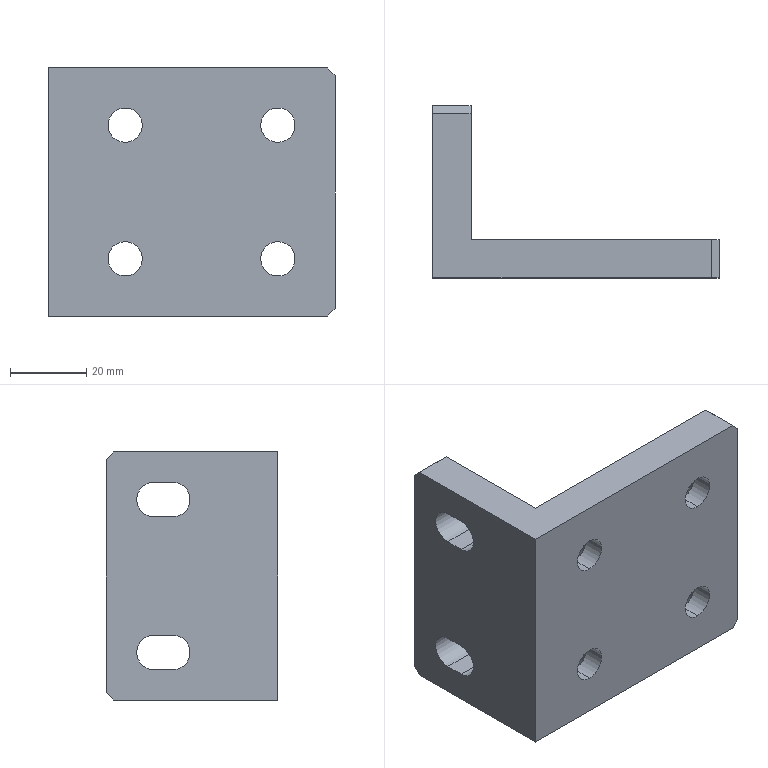Part | SolidWorks | features ICE 2, Chamfer 1, Extrusion 1, HoleWzd 1 | 1 solid | 36 faces | box 75 x 45 x 65 mm | volume 65207 mm3 | plane 16 | cylinder 12 | cone 8 | commonest cylinder face diameters 9 x12
STEP:
#1=CARTESIAN_POINT('',(22.5,0.54,-22.));
#2=VERTEX_POINT('',#1);
#3=CARTESIAN_POINT('',(22.5,0.54,-13.));
#4=VERTEX_POINT('',#3);
#5=CARTESIAN_POINT('',(22.5,0.54,-17.5));
#6=DIRECTION('',(0.,1.,0.));
#7=DIRECTION('',(0.,0.,1.));
#8=AXIS2_PLACEMENT_3D('',#5,#6,#7);
#9=CIRCLE('',#8,4.5);
#10=EDGE_CURVE('',#2,#4,#9,.T.);
#11=ORIENTED_EDGE('',*,*,#10,.F.);
#12=CARTESIAN_POINT('',(22.5,5.,-26.46));
#13=VERTEX_POINT('',#12);
#14=CARTESIAN_POINT('',(22.5,5.,-26.46));
#15=DIRECTION('',(0.,0.7071,-0.7071));
#16=VECTOR('',#15,1000.);
#17=LINE('',#14,#16);
#18=EDGE_CURVE('',#2,#13,#17,.T.);
#19=ORIENTED_EDGE('',*,*,#18,.T.);
#20=CARTESIAN_POINT('',(22.5,5.,-8.54));
#21=VERTEX_POINT('',#20);
#22=CARTESIAN_POINT('',(22.5,5.,-17.5));
#23=DIRECTION('',(0.,1.,0.));
#24=DIRECTION('',(0.,0.,1.));
#25=AXIS2_PLACEMENT_3D('',#22,#23,#24);
#26=CIRCLE('',#25,8.96);
#27=EDGE_CURVE('',#13,#21,#26,.T.);
#28=ORIENTED_EDGE('',*,*,#27,.T.);
#29=CARTESIAN_POINT('',(22.5,5.,-8.54));
#30=DIRECTION('',(0.,0.7071,0.7071));
#31=VECTOR('',#30,1000.);
#32=LINE('',#29,#31);
#33=EDGE_CURVE('',#4,#21,#32,.T.);
#34=ORIENTED_EDGE('',*,*,#33,.F.);
#35=EDGE_LOOP('',(#11,#19,#28,#34));
#36=FACE_OUTER_BOUND('',#35,.T.);
#37=CARTESIAN_POINT('',(22.5,5.,-17.5));
#38=DIRECTION('',(0.,1.,0.));
#39=DIRECTION('',(0.,0.,1.));
#40=AXIS2_PLACEMENT_3D('',#37,#38,#39);
#41=CONICAL_SURFACE('',#40,8.96,0.7854);
#42=ADVANCED_FACE('',(#36),#41,.F.);
#43=CARTESIAN_POINT('',(22.5,-5.,-22.));
#44=VERTEX_POINT('',#43);
#45=CARTESIAN_POINT('',(22.5,-5.,-13.));
#46=VERTEX_POINT('',#45);
#47=CARTESIAN_POINT('',(22.5,-5.,-17.5));
#48=DIRECTION('',(0.,1.,0.));
#49=DIRECTION('',(0.,0.,1.));
#50=AXIS2_PLACEMENT_3D('',#47,#48,#49);
#51=CIRCLE('',#50,4.5);
#52=EDGE_CURVE('',#44,#46,#51,.T.);
#53=ORIENTED_EDGE('',*,*,#52,.F.);
#54=CARTESIAN_POINT('',(22.5,5.,-22.));
#55=DIRECTION('',(0.,1.,0.));
#56=VECTOR('',#55,1000.);
#57=LINE('',#54,#56);
#58=EDGE_CURVE('',#44,#2,#57,.T.);
#59=ORIENTED_EDGE('',*,*,#58,.T.);
#60=ORIENTED_EDGE('',*,*,#10,.T.);
#61=CARTESIAN_POINT('',(22.5,5.,-13.));
#62=DIRECTION('',(0.,1.,0.));
#63=VECTOR('',#62,1000.);
#64=LINE('',#61,#63);
#65=EDGE_CURVE('',#46,#4,#64,.T.);
#66=ORIENTED_EDGE('',*,*,#65,.F.);
#67=EDGE_LOOP('',(#53,#59,#60,#66));
#68=FACE_OUTER_BOUND('',#67,.T.);
#69=CARTESIAN_POINT('',(22.5,5.,-17.5));
#70=DIRECTION('',(0.,1.,0.));
#71=DIRECTION('',(0.,0.,1.));
#72=AXIS2_PLACEMENT_3D('',#69,#70,#71);
#73=CYLINDRICAL_SURFACE('',#72,4.5);
#74=ADVANCED_FACE('',(#68),#73,.F.);
#75=CARTESIAN_POINT('',(-17.5,0.54,-22.));
#76=VERTEX_POINT('',#75);
#77=CARTESIAN_POINT('',(-17.5,0.54,-13.));
#78=VERTEX_POINT('',#77);
#79=CARTESIAN_POINT('',(-17.5,0.54,-17.5));
#80=DIRECTION('',(0.,1.,0.));
#81=DIRECTION('',(0.,0.,1.));
#82=AXIS2_PLACEMENT_3D('',#79,#80,#81);
#83=CIRCLE('',#82,4.5);
#84=EDGE_CURVE('',#76,#78,#83,.T.);
#85=ORIENTED_EDGE('',*,*,#84,.F.);
#86=CARTESIAN_POINT('',(-17.5,5.,-26.46));
#87=VERTEX_POINT('',#86);
#88=CARTESIAN_POINT('',(-17.5,5.,-26.46));
#89=DIRECTION('',(0.,0.7071,-0.7071));
#90=VECTOR('',#89,1000.);
#91=LINE('',#88,#90);
#92=EDGE_CURVE('',#76,#87,#91,.T.);
#93=ORIENTED_EDGE('',*,*,#92,.T.);
#94=CARTESIAN_POINT('',(-17.5,5.,-8.54));
#95=VERTEX_POINT('',#94);
#96=CARTESIAN_POINT('',(-17.5,5.,-17.5));
#97=DIRECTION('',(0.,1.,0.));
#98=DIRECTION('',(0.,0.,1.));
#99=AXIS2_PLACEMENT_3D('',#96,#97,#98);
#100=CIRCLE('',#99,8.96);
#101=EDGE_CURVE('',#87,#95,#100,.T.);
#102=ORIENTED_EDGE('',*,*,#101,.T.);
#103=CARTESIAN_POINT('',(-17.5,5.,-8.54));
#104=DIRECTION('',(0.,0.7071,0.7071));
#105=VECTOR('',#104,1000.);
#106=LINE('',#103,#105);
#107=EDGE_CURVE('',#78,#95,#106,.T.);
#108=ORIENTED_EDGE('',*,*,#107,.F.);
#109=EDGE_LOOP('',(#85,#93,#102,#108));
#110=FACE_OUTER_BOUND('',#109,.T.);
#111=CARTESIAN_POINT('',(-17.5,5.,-17.5));
#112=DIRECTION('',(0.,1.,0.));
#113=DIRECTION('',(0.,0.,1.));
#114=AXIS2_PLACEMENT_3D('',#111,#112,#113);
#115=CONICAL_SURFACE('',#114,8.96,0.7854);
#116=ADVANCED_FACE('',(#110),#115,.F.);
#117=CARTESIAN_POINT('',(-17.5,-5.,-22.));
#118=VERTEX_POINT('',#117);
#119=CARTESIAN_POINT('',(-17.5,-5.,-13.));
#120=VERTEX_POINT('',#119);
#121=CARTESIAN_POINT('',(-17.5,-5.,-17.5));
#122=DIRECTION('',(0.,1.,0.));
#123=DIRECTION('',(0.,0.,1.));
#124=AXIS2_PLACEMENT_3D('',#121,#122,#123);
#125=CIRCLE('',#124,4.5);
#126=EDGE_CURVE('',#118,#120,#125,.T.);
#127=ORIENTED_EDGE('',*,*,#126,.F.);
#128=CARTESIAN_POINT('',(-17.5,5.,-22.));
#129=DIRECTION('',(0.,1.,0.));
#130=VECTOR('',#129,1000.);
#131=LINE('',#128,#130);
#132=EDGE_CURVE('',#118,#76,#131,.T.);
#133=ORIENTED_EDGE('',*,*,#132,.T.);
#134=ORIENTED_EDGE('',*,*,#84,.T.);
#135=CARTESIAN_POINT('',(-17.5,5.,-13.));
#136=DIRECTION('',(0.,1.,0.));
#137=VECTOR('',#136,1000.);
#138=LINE('',#135,#137);
#139=EDGE_CURVE('',#120,#78,#138,.T.);
#140=ORIENTED_EDGE('',*,*,#139,.F.);
#141=EDGE_LOOP('',(#127,#133,#134,#140));
#142=FACE_OUTER_BOUND('',#141,.T.);
#143=CARTESIAN_POINT('',(-17.5,5.,-17.5));
#144=DIRECTION('',(0.,1.,0.));
#145=DIRECTION('',(0.,0.,1.));
#146=AXIS2_PLACEMENT_3D('',#143,#144,#145);
#147=CYLINDRICAL_SURFACE('',#146,4.5);
#148=ADVANCED_FACE('',(#142),#147,.F.);
#149=CARTESIAN_POINT('',(-17.5,0.54,13.));
#150=VERTEX_POINT('',#149);
#151=CARTESIAN_POINT('',(-17.5,0.54,22.));
#152=VERTEX_POINT('',#151);
#153=CARTESIAN_POINT('',(-17.5,0.54,17.5));
#154=DIRECTION('',(0.,1.,0.));
#155=DIRECTION('',(0.,0.,1.));
#156=AXIS2_PLACEMENT_3D('',#153,#154,#155);
#157=CIRCLE('',#156,4.5);
#158=EDGE_CURVE('',#150,#152,#157,.T.);
#159=ORIENTED_EDGE('',*,*,#158,.F.);
#160=CARTESIAN_POINT('',(-17.5,5.,8.54));
#161=VERTEX_POINT('',#160);
#162=CARTESIAN_POINT('',(-17.5,5.,8.54));
#163=DIRECTION('',(0.,0.7071,-0.7071));
#164=VECTOR('',#163,1000.);
#165=LINE('',#162,#164);
#166=EDGE_CURVE('',#150,#161,#165,.T.);
#167=ORIENTED_EDGE('',*,*,#166,.T.);
#168=CARTESIAN_POINT('',(-17.5,5.,26.46));
#169=VERTEX_POINT('',#168);
#170=CARTESIAN_POINT('',(-17.5,5.,17.5));
#171=DIRECTION('',(0.,1.,0.));
#172=DIRECTION('',(0.,0.,1.));
#173=AXIS2_PLACEMENT_3D('',#170,#171,#172);
#174=CIRCLE('',#173,8.96);
#175=EDGE_CURVE('',#161,#169,#174,.T.);
#176=ORIENTED_EDGE('',*,*,#175,.T.);
#177=CARTESIAN_POINT('',(-17.5,5.,26.46));
#178=DIRECTION('',(0.,0.7071,0.7071));
#179=VECTOR('',#178,1000.);
#180=LINE('',#177,#179);
#181=EDGE_CURVE('',#152,#169,#180,.T.);
#182=ORIENTED_EDGE('',*,*,#181,.F.);
#183=EDGE_LOOP('',(#159,#167,#176,#182));
#184=FACE_OUTER_BOUND('',#183,.T.);
#185=CARTESIAN_POINT('',(-17.5,5.,17.5));
#186=DIRECTION('',(0.,1.,0.));
#187=DIRECTION('',(0.,0.,1.));
#188=AXIS2_PLACEMENT_3D('',#185,#186,#187);
#189=CONICAL_SURFACE('',#188,8.96,0.7854);
#190=ADVANCED_FACE('',(#184),#189,.F.);
#191=CARTESIAN_POINT('',(-17.5,-5.,13.));
#192=VERTEX_POINT('',#191);
#193=CARTESIAN_POINT('',(-17.5,-5.,22.));
#194=VERTEX_POINT('',#193);
#195=CARTESIAN_POINT('',(-17.5,-5.,17.5));
#196=DIRECTION('',(0.,1.,0.));
#197=DIRECTION('',(0.,0.,1.));
#198=AXIS2_PLACEMENT_3D('',#195,#196,#197);
#199=CIRCLE('',#198,4.5);
#200=EDGE_CURVE('',#192,#194,#199,.T.);
#201=ORIENTED_EDGE('',*,*,#200,.F.);
#202=CARTESIAN_POINT('',(-17.5,5.,13.));
#203=DIRECTION('',(0.,1.,0.));
#204=VECTOR('',#203,1000.);
#205=LINE('',#202,#204);
#206=EDGE_CURVE('',#192,#150,#205,.T.);
#207=ORIENTED_EDGE('',*,*,#206,.T.);
#208=ORIENTED_EDGE('',*,*,#158,.T.);
#209=CARTESIAN_POINT('',(-17.5,5.,22.));
#210=DIRECTION('',(0.,1.,0.));
#211=VECTOR('',#210,1000.);
#212=LINE('',#209,#211);
#213=EDGE_CURVE('',#194,#152,#212,.T.);
#214=ORIENTED_EDGE('',*,*,#213,.F.);
#215=EDGE_LOOP('',(#201,#207,#208,#214));
#216=FACE_OUTER_BOUND('',#215,.T.);
#217=CARTESIAN_POINT('',(-17.5,5.,17.5));
#218=DIRECTION('',(0.,1.,0.));
#219=DIRECTION('',(0.,0.,1.));
#220=AXIS2_PLACEMENT_3D('',#217,#218,#219);
#221=CYLINDRICAL_SURFACE('',#220,4.5);
#222=ADVANCED_FACE('',(#216),#221,.F.);
#223=CARTESIAN_POINT('',(22.5,0.54,13.));
#224=VERTEX_POINT('',#223);
#225=CARTESIAN_POINT('',(22.5,0.54,22.));
#226=VERTEX_POINT('',#225);
#227=CARTESIAN_POINT('',(22.5,0.54,17.5));
#228=DIRECTION('',(0.,1.,0.));
#229=DIRECTION('',(0.,0.,1.));
#230=AXIS2_PLACEMENT_3D('',#227,#228,#229);
#231=CIRCLE('',#230,4.5);
#232=EDGE_CURVE('',#224,#226,#231,.T.);
#233=ORIENTED_EDGE('',*,*,#232,.F.);
#234=CARTESIAN_POINT('',(22.5,5.,8.54));
#235=VERTEX_POINT('',#234);
#236=CARTESIAN_POINT('',(22.5,5.,8.54));
#237=DIRECTION('',(0.,0.7071,-0.7071));
#238=VECTOR('',#237,1000.);
#239=LINE('',#236,#238);
#240=EDGE_CURVE('',#224,#235,#239,.T.);
#241=ORIENTED_EDGE('',*,*,#240,.T.);
#242=CARTESIAN_POINT('',(22.5,5.,26.46));
#243=VERTEX_POINT('',#242);
#244=CARTESIAN_POINT('',(22.5,5.,17.5));
#245=DIRECTION('',(0.,1.,0.));
#246=DIRECTION('',(0.,0.,1.));
#247=AXIS2_PLACEMENT_3D('',#244,#245,#246);
#248=CIRCLE('',#247,8.96);
#249=EDGE_CURVE('',#235,#243,#248,.T.);
#250=ORIENTED_EDGE('',*,*,#249,.T.);
#251=CARTESIAN_POINT('',(22.5,5.,26.46));
#252=DIRECTION('',(0.,0.7071,0.7071));
#253=VECTOR('',#252,1000.);
#254=LINE('',#251,#253);
#255=EDGE_CURVE('',#226,#243,#254,.T.);
#256=ORIENTED_EDGE('',*,*,#255,.F.);
#257=EDGE_LOOP('',(#233,#241,#250,#256));
#258=FACE_OUTER_BOUND('',#257,.T.);
#259=CARTESIAN_POINT('',(22.5,5.,17.5));
#260=DIRECTION('',(0.,1.,0.));
#261=DIRECTION('',(0.,0.,1.));
#262=AXIS2_PLACEMENT_3D('',#259,#260,#261);
#263=CONICAL_SURFACE('',#262,8.96,0.7854);
#264=ADVANCED_FACE('',(#258),#263,.F.);
#265=CARTESIAN_POINT('',(22.5,-5.,13.));
#266=VERTEX_POINT('',#265);
#267=CARTESIAN_POINT('',(22.5,-5.,22.));
#268=VERTEX_POINT('',#267);
#269=CARTESIAN_POINT('',(22.5,-5.,17.5));
#270=DIRECTION('',(0.,1.,0.));
#271=DIRECTION('',(0.,0.,1.));
#272=AXIS2_PLACEMENT_3D('',#269,#270,#271);
#273=CIRCLE('',#272,4.5);
#274=EDGE_CURVE('',#266,#268,#273,.T.);
#275=ORIENTED_EDGE('',*,*,#274,.F.);
#276=CARTESIAN_POINT('',(22.5,5.,13.));
#277=DIRECTION('',(0.,1.,0.));
#278=VECTOR('',#277,1000.);
#279=LINE('',#276,#278);
#280=EDGE_CURVE('',#266,#224,#279,.T.);
#281=ORIENTED_EDGE('',*,*,#280,.T.);
#282=ORIENTED_EDGE('',*,*,#232,.T.);
#283=CARTESIAN_POINT('',(22.5,5.,22.));
#284=DIRECTION('',(0.,1.,0.));
#285=VECTOR('',#284,1000.);
#286=LINE('',#283,#285);
#287=EDGE_CURVE('',#268,#226,#286,.T.);
#288=ORIENTED_EDGE('',*,*,#287,.F.);
#289=EDGE_LOOP('',(#275,#281,#282,#288));
#290=FACE_OUTER_BOUND('',#289,.T.);
#291=CARTESIAN_POINT('',(22.5,5.,17.5));
#292=DIRECTION('',(0.,1.,0.));
#293=DIRECTION('',(0.,0.,1.));
#294=AXIS2_PLACEMENT_3D('',#291,#292,#293);
#295=CYLINDRICAL_SURFACE('',#294,4.5);
#296=ADVANCED_FACE('',(#290),#295,.F.);
#297=CARTESIAN_POINT('',(37.5,5.,30.5));
#298=VERTEX_POINT('',#297);
#299=CARTESIAN_POINT('',(37.5,5.,-30.5));
#300=VERTEX_POINT('',#299);
#301=CARTESIAN_POINT('',(37.5,5.,-32.5));
#302=DIRECTION('',(0.,0.,-1.));
#303=VECTOR('',#302,1000.);
#304=LINE('',#301,#303);
#305=EDGE_CURVE('',#298,#300,#304,.T.);
#306=ORIENTED_EDGE('',*,*,#305,.F.);
#307=CARTESIAN_POINT('',(37.5,-5.,30.5));
#308=VERTEX_POINT('',#307);
#309=CARTESIAN_POINT('',(37.5,5.,30.5));
#310=DIRECTION('',(0.,-1.,0.));
#311=VECTOR('',#310,1000.);
#312=LINE('',#309,#311);
#313=EDGE_CURVE('',#298,#308,#312,.T.);
#314=ORIENTED_EDGE('',*,*,#313,.T.);
#315=CARTESIAN_POINT('',(37.5,-5.,-30.5));
#316=VERTEX_POINT('',#315);
#317=CARTESIAN_POINT('',(37.5,-5.,-32.5));
#318=DIRECTION('',(0.,0.,-1.));
#319=VECTOR('',#318,1000.);
#320=LINE('',#317,#319);
#321=EDGE_CURVE('',#308,#316,#320,.T.);
#322=ORIENTED_EDGE('',*,*,#321,.T.);
#323=CARTESIAN_POINT('',(37.5,5.,-30.5));
#324=DIRECTION('',(0.,1.,0.));
#325=VECTOR('',#324,1000.);
#326=LINE('',#323,#325);
#327=EDGE_CURVE('',#316,#300,#326,.T.);
#328=ORIENTED_EDGE('',*,*,#327,.T.);
#329=EDGE_LOOP('',(#306,#314,#322,#328));
#330=FACE_OUTER_BOUND('',#329,.T.);
#331=CARTESIAN_POINT('',(37.5,5.,-32.5));
#332=DIRECTION('',(-1.,0.,0.));
#333=DIRECTION('',(0.,0.,1.));
#334=AXIS2_PLACEMENT_3D('',#331,#332,#333);
#335=PLANE('',#334);
#336=ADVANCED_FACE('',(#330),#335,.F.);
#337=CARTESIAN_POINT('',(35.5,5.,-32.5));
#338=VERTEX_POINT('',#337);
#339=CARTESIAN_POINT('',(-27.5,5.,-32.5));
#340=VERTEX_POINT('',#339);
#341=CARTESIAN_POINT('',(-37.5,5.,-32.5));
#342=DIRECTION('',(-1.,0.,0.));
#343=VECTOR('',#342,1000.);
#344=LINE('',#341,#343);
#345=EDGE_CURVE('',#338,#340,#344,.T.);
#346=ORIENTED_EDGE('',*,*,#345,.F.);
#347=CARTESIAN_POINT('',(35.5,-5.,-32.5));
#348=VERTEX_POINT('',#347);
#349=CARTESIAN_POINT('',(35.5,5.,-32.5));
#350=DIRECTION('',(0.,-1.,0.));
#351=VECTOR('',#350,1000.);
#352=LINE('',#349,#351);
#353=EDGE_CURVE('',#338,#348,#352,.T.);
#354=ORIENTED_EDGE('',*,*,#353,.T.);
#355=CARTESIAN_POINT('',(-37.5,-5.,-32.5));
#356=VERTEX_POINT('',#355);
#357=CARTESIAN_POINT('',(-37.5,-5.,-32.5));
#358=DIRECTION('',(-1.,0.,0.));
#359=VECTOR('',#358,1000.);
#360=LINE('',#357,#359);
#361=EDGE_CURVE('',#348,#356,#360,.T.);
#362=ORIENTED_EDGE('',*,*,#361,.T.);
#363=CARTESIAN_POINT('',(-37.5,38.,-32.5));
#364=VERTEX_POINT('',#363);
#365=CARTESIAN_POINT('',(-37.5,5.,-32.5));
#366=DIRECTION('',(0.,-1.,0.));
#367=VECTOR('',#366,1000.);
#368=LINE('',#365,#367);
#369=EDGE_CURVE('',#364,#356,#368,.T.);
#370=ORIENTED_EDGE('',*,*,#369,.F.);
#371=CARTESIAN_POINT('',(-27.5,38.,-32.5));
#372=VERTEX_POINT('',#371);
#373=CARTESIAN_POINT('',(-37.5,38.,-32.5));
#374=DIRECTION('',(1.,0.,0.));
#375=VECTOR('',#374,1000.);
#376=LINE('',#373,#375);
#377=EDGE_CURVE('',#364,#372,#376,.T.);
#378=ORIENTED_EDGE('',*,*,#377,.T.);
#379=CARTESIAN_POINT('',(-27.5,40.,-32.5));
#380=DIRECTION('',(0.,-1.,0.));
#381=VECTOR('',#380,1000.);
#382=LINE('',#379,#381);
#383=EDGE_CURVE('',#372,#340,#382,.T.);
#384=ORIENTED_EDGE('',*,*,#383,.T.);
#385=EDGE_LOOP('',(#346,#354,#362,#370,#378,#384));
#386=FACE_OUTER_BOUND('',#385,.T.);
#387=CARTESIAN_POINT('',(-37.5,5.,-32.5));
#388=DIRECTION('',(0.,0.,1.));
#389=DIRECTION('',(1.,0.,0.));
#390=AXIS2_PLACEMENT_3D('',#387,#388,#389);
#391=PLANE('',#390);
#392=ADVANCED_FACE('',(#386),#391,.F.);
#393=CARTESIAN_POINT('',(-37.5,22.5,15.5));
#394=VERTEX_POINT('',#393);
#395=CARTESIAN_POINT('',(-37.5,27.5,15.5));
#396=VERTEX_POINT('',#395);
#397=CARTESIAN_POINT('',(-37.5,5.,15.5));
#398=DIRECTION('',(0.,1.,0.));
#399=VECTOR('',#398,1000.);
#400=LINE('',#397,#399);
#401=EDGE_CURVE('',#394,#396,#400,.T.);
#402=ORIENTED_EDGE('',*,*,#401,.T.);
#403=CARTESIAN_POINT('',(-37.5,27.5,24.5));
#404=VERTEX_POINT('',#403);
#405=CARTESIAN_POINT('',(-37.5,27.5,20.));
#406=DIRECTION('',(1.,0.,0.));
#407=DIRECTION('',(0.,0.,-1.));
#408=AXIS2_PLACEMENT_3D('',#405,#406,#407);
#409=CIRCLE('',#408,4.5);
#410=EDGE_CURVE('',#396,#404,#409,.T.);
#411=ORIENTED_EDGE('',*,*,#410,.T.);
#412=CARTESIAN_POINT('',(-37.5,22.5,24.5));
#413=VERTEX_POINT('',#412);
#414=CARTESIAN_POINT('',(-37.5,5.,24.5));
#415=DIRECTION('',(0.,-1.,0.));
#416=VECTOR('',#415,1000.);
#417=LINE('',#414,#416);
#418=EDGE_CURVE('',#404,#413,#417,.T.);
#419=ORIENTED_EDGE('',*,*,#418,.T.);
#420=CARTESIAN_POINT('',(-37.5,22.5,20.));
#421=DIRECTION('',(1.,0.,0.));
#422=DIRECTION('',(0.,0.,-1.));
#423=AXIS2_PLACEMENT_3D('',#420,#421,#422);
#424=CIRCLE('',#423,4.5);
#425=EDGE_CURVE('',#413,#394,#424,.T.);
#426=ORIENTED_EDGE('',*,*,#425,.T.);
#427=EDGE_LOOP('',(#402,#411,#419,#426));
#428=FACE_BOUND('',#427,.T.);
#429=CARTESIAN_POINT('',(-37.5,22.5,-24.5));
#430=VERTEX_POINT('',#429);
#431=CARTESIAN_POINT('',(-37.5,27.5,-24.5));
#432=VERTEX_POINT('',#431);
#433=CARTESIAN_POINT('',(-37.5,5.,-24.5));
#434=DIRECTION('',(0.,1.,0.));
#435=VECTOR('',#434,1000.);
#436=LINE('',#433,#435);
#437=EDGE_CURVE('',#430,#432,#436,.T.);
#438=ORIENTED_EDGE('',*,*,#437,.T.);
#439=CARTESIAN_POINT('',(-37.5,27.5,-15.5));
#440=VERTEX_POINT('',#439);
#441=CARTESIAN_POINT('',(-37.5,27.5,-20.));
#442=DIRECTION('',(1.,0.,0.));
#443=DIRECTION('',(0.,0.,-1.));
#444=AXIS2_PLACEMENT_3D('',#441,#442,#443);
#445=CIRCLE('',#444,4.5);
#446=EDGE_CURVE('',#432,#440,#445,.T.);
#447=ORIENTED_EDGE('',*,*,#446,.T.);
#448=CARTESIAN_POINT('',(-37.5,22.5,-15.5));
#449=VERTEX_POINT('',#448);
#450=CARTESIAN_POINT('',(-37.5,5.,-15.5));
#451=DIRECTION('',(0.,-1.,0.));
#452=VECTOR('',#451,1000.);
#453=LINE('',#450,#452);
#454=EDGE_CURVE('',#440,#449,#453,.T.);
#455=ORIENTED_EDGE('',*,*,#454,.T.);
#456=CARTESIAN_POINT('',(-37.5,22.5,-20.));
#457=DIRECTION('',(1.,0.,0.));
#458=DIRECTION('',(0.,0.,-1.));
#459=AXIS2_PLACEMENT_3D('',#456,#457,#458);
#460=CIRCLE('',#459,4.5);
#461=EDGE_CURVE('',#449,#430,#460,.T.);
#462=ORIENTED_EDGE('',*,*,#461,.T.);
#463=EDGE_LOOP('',(#438,#447,#455,#462));
#464=FACE_BOUND('',#463,.T.);
#465=CARTESIAN_POINT('',(-37.5,40.,-30.5));
#466=VERTEX_POINT('',#465);
#467=CARTESIAN_POINT('',(-37.5,40.,30.5));
#468=VERTEX_POINT('',#467);
#469=CARTESIAN_POINT('',(-37.5,40.,-32.5));
#470=DIRECTION('',(0.,0.,1.));
#471=VECTOR('',#470,1000.);
#472=LINE('',#469,#471);
#473=EDGE_CURVE('',#466,#468,#472,.T.);
#474=ORIENTED_EDGE('',*,*,#473,.F.);
#475=CARTESIAN_POINT('',(-37.5,38.,-32.5));
#476=DIRECTION('',(0.,-0.7071,-0.7071));
#477=VECTOR('',#476,1000.);
#478=LINE('',#475,#477);
#479=EDGE_CURVE('',#466,#364,#478,.T.);
#480=ORIENTED_EDGE('',*,*,#479,.T.);
#481=ORIENTED_EDGE('',*,*,#369,.T.);
#482=CARTESIAN_POINT('',(-37.5,-5.,32.5));
#483=VERTEX_POINT('',#482);
#484=CARTESIAN_POINT('',(-37.5,-5.,-32.5));
#485=DIRECTION('',(0.,0.,1.));
#486=VECTOR('',#485,1000.);
#487=LINE('',#484,#486);
#488=EDGE_CURVE('',#356,#483,#487,.T.);
#489=ORIENTED_EDGE('',*,*,#488,.T.);
#490=CARTESIAN_POINT('',(-37.5,38.,32.5));
#491=VERTEX_POINT('',#490);
#492=CARTESIAN_POINT('',(-37.5,5.,32.5));
#493=DIRECTION('',(0.,-1.,0.));
#494=VECTOR('',#493,1000.);
#495=LINE('',#492,#494);
#496=EDGE_CURVE('',#491,#483,#495,.T.);
#497=ORIENTED_EDGE('',*,*,#496,.F.);
#498=CARTESIAN_POINT('',(-37.5,40.,30.5));
#499=DIRECTION('',(0.,0.7071,-0.7071));
#500=VECTOR('',#499,1000.);
#501=LINE('',#498,#500);
#502=EDGE_CURVE('',#491,#468,#501,.T.);
#503=ORIENTED_EDGE('',*,*,#502,.T.);
#504=EDGE_LOOP('',(#474,#480,#481,#489,#497,#503));
#505=FACE_OUTER_BOUND('',#504,.T.);
#506=CARTESIAN_POINT('',(-37.5,5.,-32.5));
#507=DIRECTION('',(1.,0.,0.));
#508=DIRECTION('',(0.,0.,-1.));
#509=AXIS2_PLACEMENT_3D('',#506,#507,#508);
#510=PLANE('',#509);
#511=ADVANCED_FACE('',(#428,#464,#505),#510,.F.);
#512=CARTESIAN_POINT('',(35.5,-5.,32.5));
#513=VERTEX_POINT('',#512);
#514=CARTESIAN_POINT('',(-37.5,-5.,32.5));
#515=DIRECTION('',(1.,0.,0.));
#516=VECTOR('',#515,1000.);
#517=LINE('',#514,#516);
#518=EDGE_CURVE('',#483,#513,#517,.T.);
#519=ORIENTED_EDGE('',*,*,#518,.T.);
#520=CARTESIAN_POINT('',(35.5,5.,32.5));
#521=VERTEX_POINT('',#520);
#522=CARTESIAN_POINT('',(35.5,5.,32.5));
#523=DIRECTION('',(0.,1.,0.));
#524=VECTOR('',#523,1000.);
#525=LINE('',#522,#524);
#526=EDGE_CURVE('',#513,#521,#525,.T.);
#527=ORIENTED_EDGE('',*,*,#526,.T.);
#528=CARTESIAN_POINT('',(-27.5,5.,32.5));
#529=VERTEX_POINT('',#528);
#530=CARTESIAN_POINT('',(-37.5,5.,32.5));
#531=DIRECTION('',(1.,0.,0.));
#532=VECTOR('',#531,1000.);
#533=LINE('',#530,#532);
#534=EDGE_CURVE('',#529,#521,#533,.T.);
#535=ORIENTED_EDGE('',*,*,#534,.F.);
#536=CARTESIAN_POINT('',(-27.5,38.,32.5));
#537=VERTEX_POINT('',#536);
#538=CARTESIAN_POINT('',(-27.5,40.,32.5));
#539=DIRECTION('',(0.,-1.,0.));
#540=VECTOR('',#539,1000.);
#541=LINE('',#538,#540);
#542=EDGE_CURVE('',#537,#529,#541,.T.);
#543=ORIENTED_EDGE('',*,*,#542,.F.);
#544=CARTESIAN_POINT('',(-37.5,38.,32.5));
#545=DIRECTION('',(-1.,0.,0.));
#546=VECTOR('',#545,1000.);
#547=LINE('',#544,#546);
#548=EDGE_CURVE('',#537,#491,#547,.T.);
#549=ORIENTED_EDGE('',*,*,#548,.T.);
#550=ORIENTED_EDGE('',*,*,#496,.T.);
#551=EDGE_LOOP('',(#519,#527,#535,#543,#549,#550));
#552=FACE_OUTER_BOUND('',#551,.T.);
#553=CARTESIAN_POINT('',(-37.5,5.,32.5));
#554=DIRECTION('',(0.,0.,-1.));
#555=DIRECTION('',(-1.,0.,0.));
#556=AXIS2_PLACEMENT_3D('',#553,#554,#555);
#557=PLANE('',#556);
#558=ADVANCED_FACE('',(#552),#557,.F.);
#559=CARTESIAN_POINT('',(22.5,5.,-17.5));
#560=DIRECTION('',(0.,1.,0.));
#561=DIRECTION('',(0.,0.,1.));
#562=AXIS2_PLACEMENT_3D('',#559,#560,#561);
#563=CIRCLE('',#562,8.96);
#564=EDGE_CURVE('',#21,#13,#563,.T.);
#565=ORIENTED_EDGE('',*,*,#564,.F.);
#566=ORIENTED_EDGE('',*,*,#27,.F.);
#567=EDGE_LOOP('',(#565,#566));
#568=FACE_BOUND('',#567,.T.);
#569=CARTESIAN_POINT('',(-17.5,5.,-17.5));
#570=DIRECTION('',(0.,1.,0.));
#571=DIRECTION('',(0.,0.,1.));
#572=AXIS2_PLACEMENT_3D('',#569,#570,#571);
#573=CIRCLE('',#572,8.96);
#574=EDGE_CURVE('',#95,#87,#573,.T.);
#575=ORIENTED_EDGE('',*,*,#574,.F.);
#576=ORIENTED_EDGE('',*,*,#101,.F.);
#577=EDGE_LOOP('',(#575,#576));
#578=FACE_BOUND('',#577,.T.);
#579=CARTESIAN_POINT('',(-17.5,5.,17.5));
#580=DIRECTION('',(0.,1.,0.));
#581=DIRECTION('',(0.,0.,1.));
#582=AXIS2_PLACEMENT_3D('',#579,#580,#581);
#583=CIRCLE('',#582,8.96);
#584=EDGE_CURVE('',#169,#161,#583,.T.);
#585=ORIENTED_EDGE('',*,*,#584,.F.);
#586=ORIENTED_EDGE('',*,*,#175,.F.);
#587=EDGE_LOOP('',(#585,#586));
#588=FACE_BOUND('',#587,.T.);
#589=CARTESIAN_POINT('',(22.5,5.,17.5));
#590=DIRECTION('',(0.,1.,0.));
#591=DIRECTION('',(0.,0.,1.));
#592=AXIS2_PLACEMENT_3D('',#589,#590,#591);
#593=CIRCLE('',#592,8.96);
#594=EDGE_CURVE('',#243,#235,#593,.T.);
#595=ORIENTED_EDGE('',*,*,#594,.F.);
#596=ORIENTED_EDGE('',*,*,#249,.F.);
#597=EDGE_LOOP('',(#595,#596));
#598=FACE_BOUND('',#597,.T.);
#599=ORIENTED_EDGE('',*,*,#534,.T.);
#600=CARTESIAN_POINT('',(34.,5.,34.));
#601=DIRECTION('',(0.7071,0.,-0.7071));
#602=VECTOR('',#601,1000.);
#603=LINE('',#600,#602);
#604=EDGE_CURVE('',#521,#298,#603,.T.);
#605=ORIENTED_EDGE('',*,*,#604,.T.);
#606=ORIENTED_EDGE('',*,*,#305,.T.);
#607=CARTESIAN_POINT('',(34.,5.,-34.));
#608=DIRECTION('',(-0.7071,0.,-0.7071));
#609=VECTOR('',#608,1000.);
#610=LINE('',#607,#609);
#611=EDGE_CURVE('',#300,#338,#610,.T.);
#612=ORIENTED_EDGE('',*,*,#611,.T.);
#613=ORIENTED_EDGE('',*,*,#345,.T.);
#614=CARTESIAN_POINT('',(-27.5,5.,0.));
#615=DIRECTION('',(0.,0.,-1.));
#616=VECTOR('',#615,1000.);
#617=LINE('',#614,#616);
#618=EDGE_CURVE('',#529,#340,#617,.T.);
#619=ORIENTED_EDGE('',*,*,#618,.F.);
#620=EDGE_LOOP('',(#599,#605,#606,#612,#613,#619));
#621=FACE_OUTER_BOUND('',#620,.T.);
#622=CARTESIAN_POINT('',(0.,5.,0.));
#623=DIRECTION('',(0.,1.,0.));
#624=DIRECTION('',(0.,0.,1.));
#625=AXIS2_PLACEMENT_3D('',#622,#623,#624);
#626=PLANE('',#625);
#627=ADVANCED_FACE('',(#568,#578,#588,#598,#621),#626,.T.);
#628=CARTESIAN_POINT('',(22.5,-5.,-17.5));
#629=DIRECTION('',(0.,1.,0.));
#630=DIRECTION('',(0.,0.,1.));
#631=AXIS2_PLACEMENT_3D('',#628,#629,#630);
#632=CIRCLE('',#631,4.5);
#633=EDGE_CURVE('',#46,#44,#632,.T.);
#634=ORIENTED_EDGE('',*,*,#633,.T.);
#635=ORIENTED_EDGE('',*,*,#52,.T.);
#636=EDGE_LOOP('',(#634,#635));
#637=FACE_BOUND('',#636,.T.);
#638=CARTESIAN_POINT('',(-17.5,-5.,-17.5));
#639=DIRECTION('',(0.,1.,0.));
#640=DIRECTION('',(0.,0.,1.));
#641=AXIS2_PLACEMENT_3D('',#638,#639,#640);
#642=CIRCLE('',#641,4.5);
#643=EDGE_CURVE('',#120,#118,#642,.T.);
#644=ORIENTED_EDGE('',*,*,#643,.T.);
#645=ORIENTED_EDGE('',*,*,#126,.T.);
#646=EDGE_LOOP('',(#644,#645));
#647=FACE_BOUND('',#646,.T.);
#648=CARTESIAN_POINT('',(-17.5,-5.,17.5));
#649=DIRECTION('',(0.,1.,0.));
#650=DIRECTION('',(0.,0.,1.));
#651=AXIS2_PLACEMENT_3D('',#648,#649,#650);
#652=CIRCLE('',#651,4.5);
#653=EDGE_CURVE('',#194,#192,#652,.T.);
#654=ORIENTED_EDGE('',*,*,#653,.T.);
#655=ORIENTED_EDGE('',*,*,#200,.T.);
#656=EDGE_LOOP('',(#654,#655));
#657=FACE_BOUND('',#656,.T.);
#658=CARTESIAN_POINT('',(22.5,-5.,17.5));
#659=DIRECTION('',(0.,1.,0.));
#660=DIRECTION('',(0.,0.,1.));
#661=AXIS2_PLACEMENT_3D('',#658,#659,#660);
#662=CIRCLE('',#661,4.5);
#663=EDGE_CURVE('',#268,#266,#662,.T.);
#664=ORIENTED_EDGE('',*,*,#663,.T.);
#665=ORIENTED_EDGE('',*,*,#274,.T.);
#666=EDGE_LOOP('',(#664,#665));
#667=FACE_BOUND('',#666,.T.);
#668=ORIENTED_EDGE('',*,*,#321,.F.);
#669=CARTESIAN_POINT('',(37.5,-5.,30.5));
#670=DIRECTION('',(-0.7071,0.,0.7071));
#671=VECTOR('',#670,1000.);
#672=LINE('',#669,#671);
#673=EDGE_CURVE('',#308,#513,#672,.T.);
#674=ORIENTED_EDGE('',*,*,#673,.T.);
#675=ORIENTED_EDGE('',*,*,#518,.F.);
#676=ORIENTED_EDGE('',*,*,#488,.F.);
#677=ORIENTED_EDGE('',*,*,#361,.F.);
#678=CARTESIAN_POINT('',(35.5,-5.,-32.5));
#679=DIRECTION('',(0.7071,0.,0.7071));
#680=VECTOR('',#679,1000.);
#681=LINE('',#678,#680);
#682=EDGE_CURVE('',#348,#316,#681,.T.);
#683=ORIENTED_EDGE('',*,*,#682,.T.);
#684=EDGE_LOOP('',(#668,#674,#675,#676,#677,#683));
#685=FACE_OUTER_BOUND('',#684,.T.);
#686=CARTESIAN_POINT('',(0.,-5.,0.));
#687=DIRECTION('',(0.,1.,0.));
#688=DIRECTION('',(0.,0.,1.));
#689=AXIS2_PLACEMENT_3D('',#686,#687,#688);
#690=PLANE('',#689);
#691=ADVANCED_FACE('',(#637,#647,#657,#667,#685),#690,.F.);
#692=CARTESIAN_POINT('',(-27.5,27.5,15.5));
#693=VERTEX_POINT('',#692);
#694=CARTESIAN_POINT('',(-27.5,27.5,24.5));
#695=VERTEX_POINT('',#694);
#696=CARTESIAN_POINT('',(-27.5,27.5,20.));
#697=DIRECTION('',(1.,0.,0.));
#698=DIRECTION('',(0.,0.,1.));
#699=AXIS2_PLACEMENT_3D('',#696,#697,#698);
#700=CIRCLE('',#699,4.5);
#701=EDGE_CURVE('',#693,#695,#700,.T.);
#702=ORIENTED_EDGE('',*,*,#701,.F.);
#703=CARTESIAN_POINT('',(-27.5,22.5,15.5));
#704=VERTEX_POINT('',#703);
#705=CARTESIAN_POINT('',(-27.5,27.5,15.5));
#706=DIRECTION('',(0.,1.,0.));
#707=VECTOR('',#706,1000.);
#708=LINE('',#705,#707);
#709=EDGE_CURVE('',#704,#693,#708,.T.);
#710=ORIENTED_EDGE('',*,*,#709,.F.);
#711=CARTESIAN_POINT('',(-27.5,22.5,24.5));
#712=VERTEX_POINT('',#711);
#713=CARTESIAN_POINT('',(-27.5,22.5,20.));
#714=DIRECTION('',(1.,0.,0.));
#715=DIRECTION('',(0.,0.,1.));
#716=AXIS2_PLACEMENT_3D('',#713,#714,#715);
#717=CIRCLE('',#716,4.5);
#718=EDGE_CURVE('',#712,#704,#717,.T.);
#719=ORIENTED_EDGE('',*,*,#718,.F.);
#720=CARTESIAN_POINT('',(-27.5,27.5,24.5));
#721=DIRECTION('',(0.,-1.,0.));
#722=VECTOR('',#721,1000.);
#723=LINE('',#720,#722);
#724=EDGE_CURVE('',#695,#712,#723,.T.);
#725=ORIENTED_EDGE('',*,*,#724,.F.);
#726=EDGE_LOOP('',(#702,#710,#719,#725));
#727=FACE_BOUND('',#726,.T.);
#728=CARTESIAN_POINT('',(-27.5,27.5,-24.5));
#729=VERTEX_POINT('',#728);
#730=CARTESIAN_POINT('',(-27.5,27.5,-15.5));
#731=VERTEX_POINT('',#730);
#732=CARTESIAN_POINT('',(-27.5,27.5,-20.));
#733=DIRECTION('',(1.,0.,0.));
#734=DIRECTION('',(0.,0.,-1.));
#735=AXIS2_PLACEMENT_3D('',#732,#733,#734);
#736=CIRCLE('',#735,4.5);
#737=EDGE_CURVE('',#729,#731,#736,.T.);
#738=ORIENTED_EDGE('',*,*,#737,.F.);
#739=CARTESIAN_POINT('',(-27.5,22.5,-24.5));
#740=VERTEX_POINT('',#739);
#741=CARTESIAN_POINT('',(-27.5,27.5,-24.5));
#742=DIRECTION('',(0.,1.,0.));
#743=VECTOR('',#742,1000.);
#744=LINE('',#741,#743);
#745=EDGE_CURVE('',#740,#729,#744,.T.);
#746=ORIENTED_EDGE('',*,*,#745,.F.);
#747=CARTESIAN_POINT('',(-27.5,22.5,-15.5));
#748=VERTEX_POINT('',#747);
#749=CARTESIAN_POINT('',(-27.5,22.5,-20.));
#750=DIRECTION('',(1.,0.,0.));
#751=DIRECTION('',(0.,0.,-1.));
#752=AXIS2_PLACEMENT_3D('',#749,#750,#751);
#753=CIRCLE('',#752,4.5);
#754=EDGE_CURVE('',#748,#740,#753,.T.);
#755=ORIENTED_EDGE('',*,*,#754,.F.);
#756=CARTESIAN_POINT('',(-27.5,27.5,-15.5));
#757=DIRECTION('',(0.,-1.,0.));
#758=VECTOR('',#757,1000.);
#759=LINE('',#756,#758);
#760=EDGE_CURVE('',#731,#748,#759,.T.);
#761=ORIENTED_EDGE('',*,*,#760,.F.);
#762=EDGE_LOOP('',(#738,#746,#755,#761));
#763=FACE_BOUND('',#762,.T.);
#764=ORIENTED_EDGE('',*,*,#383,.F.);
#765=CARTESIAN_POINT('',(-27.5,40.,-30.5));
#766=VERTEX_POINT('',#765);
#767=CARTESIAN_POINT('',(-27.5,39.,-31.5));
#768=DIRECTION('',(0.,0.7071,0.7071));
#769=VECTOR('',#768,1000.);
#770=LINE('',#767,#769);
#771=EDGE_CURVE('',#372,#766,#770,.T.);
#772=ORIENTED_EDGE('',*,*,#771,.T.);
#773=CARTESIAN_POINT('',(-27.5,40.,30.5));
#774=VERTEX_POINT('',#773);
#775=CARTESIAN_POINT('',(-27.5,40.,-32.5));
#776=DIRECTION('',(0.,0.,1.));
#777=VECTOR('',#776,1000.);
#778=LINE('',#775,#777);
#779=EDGE_CURVE('',#766,#774,#778,.T.);
#780=ORIENTED_EDGE('',*,*,#779,.T.);
#781=CARTESIAN_POINT('',(-27.5,71.5,-1.));
#782=DIRECTION('',(0.,-0.7071,0.7071));
#783=VECTOR('',#782,1000.);
#784=LINE('',#781,#783);
#785=EDGE_CURVE('',#774,#537,#784,.T.);
#786=ORIENTED_EDGE('',*,*,#785,.T.);
#787=ORIENTED_EDGE('',*,*,#542,.T.);
#788=ORIENTED_EDGE('',*,*,#618,.T.);
#789=EDGE_LOOP('',(#764,#772,#780,#786,#787,#788));
#790=FACE_OUTER_BOUND('',#789,.T.);
#791=CARTESIAN_POINT('',(-27.5,40.,-32.5));
#792=DIRECTION('',(1.,0.,0.));
#793=DIRECTION('',(0.,0.,-1.));
#794=AXIS2_PLACEMENT_3D('',#791,#792,#793);
#795=PLANE('',#794);
#796=ADVANCED_FACE('',(#727,#763,#790),#795,.T.);
#797=ORIENTED_EDGE('',*,*,#779,.F.);
#798=CARTESIAN_POINT('',(0.,40.,-30.5));
#799=DIRECTION('',(-1.,0.,0.));
#800=VECTOR('',#799,1000.);
#801=LINE('',#798,#800);
#802=EDGE_CURVE('',#766,#466,#801,.T.);
#803=ORIENTED_EDGE('',*,*,#802,.T.);
#804=ORIENTED_EDGE('',*,*,#473,.T.);
#805=CARTESIAN_POINT('',(0.,40.,30.5));
#806=DIRECTION('',(1.,0.,0.));
#807=VECTOR('',#806,1000.);
#808=LINE('',#805,#807);
#809=EDGE_CURVE('',#468,#774,#808,.T.);
#810=ORIENTED_EDGE('',*,*,#809,.T.);
#811=EDGE_LOOP('',(#797,#803,#804,#810));
#812=FACE_OUTER_BOUND('',#811,.T.);
#813=CARTESIAN_POINT('',(0.,40.,0.));
#814=DIRECTION('',(0.,-1.,0.));
#815=DIRECTION('',(0.,0.,-1.));
#816=AXIS2_PLACEMENT_3D('',#813,#814,#815);
#817=PLANE('',#816);
#818=ADVANCED_FACE('',(#812),#817,.F.);
#819=ORIENTED_EDGE('',*,*,#280,.F.);
#820=ORIENTED_EDGE('',*,*,#663,.F.);
#821=ORIENTED_EDGE('',*,*,#287,.T.);
#822=CARTESIAN_POINT('',(22.5,0.54,17.5));
#823=DIRECTION('',(0.,1.,0.));
#824=DIRECTION('',(0.,0.,1.));
#825=AXIS2_PLACEMENT_3D('',#822,#823,#824);
#826=CIRCLE('',#825,4.5);
#827=EDGE_CURVE('',#226,#224,#826,.T.);
#828=ORIENTED_EDGE('',*,*,#827,.T.);
#829=EDGE_LOOP('',(#819,#820,#821,#828));
#830=FACE_OUTER_BOUND('',#829,.T.);
#831=CARTESIAN_POINT('',(22.5,5.,17.5));
#832=DIRECTION('',(0.,1.,0.));
#833=DIRECTION('',(0.,0.,1.));
#834=AXIS2_PLACEMENT_3D('',#831,#832,#833);
#835=CYLINDRICAL_SURFACE('',#834,4.5);
#836=ADVANCED_FACE('',(#830),#835,.F.);
#837=ORIENTED_EDGE('',*,*,#240,.F.);
#838=ORIENTED_EDGE('',*,*,#827,.F.);
#839=ORIENTED_EDGE('',*,*,#255,.T.);
#840=ORIENTED_EDGE('',*,*,#594,.T.);
#841=EDGE_LOOP('',(#837,#838,#839,#840));
#842=FACE_OUTER_BOUND('',#841,.T.);
#843=CARTESIAN_POINT('',(22.5,5.,17.5));
#844=DIRECTION('',(0.,1.,0.));
#845=DIRECTION('',(0.,0.,1.));
#846=AXIS2_PLACEMENT_3D('',#843,#844,#845);
#847=CONICAL_SURFACE('',#846,8.96,0.7854);
#848=ADVANCED_FACE('',(#842),#847,.F.);
#849=ORIENTED_EDGE('',*,*,#206,.F.);
#850=ORIENTED_EDGE('',*,*,#653,.F.);
#851=ORIENTED_EDGE('',*,*,#213,.T.);
#852=CARTESIAN_POINT('',(-17.5,0.54,17.5));
#853=DIRECTION('',(0.,1.,0.));
#854=DIRECTION('',(0.,0.,1.));
#855=AXIS2_PLACEMENT_3D('',#852,#853,#854);
#856=CIRCLE('',#855,4.5);
#857=EDGE_CURVE('',#152,#150,#856,.T.);
#858=ORIENTED_EDGE('',*,*,#857,.T.);
#859=EDGE_LOOP('',(#849,#850,#851,#858));
#860=FACE_OUTER_BOUND('',#859,.T.);
#861=CARTESIAN_POINT('',(-17.5,5.,17.5));
#862=DIRECTION('',(0.,1.,0.));
#863=DIRECTION('',(0.,0.,1.));
#864=AXIS2_PLACEMENT_3D('',#861,#862,#863);
#865=CYLINDRICAL_SURFACE('',#864,4.5);
#866=ADVANCED_FACE('',(#860),#865,.F.);
#867=ORIENTED_EDGE('',*,*,#166,.F.);
#868=ORIENTED_EDGE('',*,*,#857,.F.);
#869=ORIENTED_EDGE('',*,*,#181,.T.);
#870=ORIENTED_EDGE('',*,*,#584,.T.);
#871=EDGE_LOOP('',(#867,#868,#869,#870));
#872=FACE_OUTER_BOUND('',#871,.T.);
#873=CARTESIAN_POINT('',(-17.5,5.,17.5));
#874=DIRECTION('',(0.,1.,0.));
#875=DIRECTION('',(0.,0.,1.));
#876=AXIS2_PLACEMENT_3D('',#873,#874,#875);
#877=CONICAL_SURFACE('',#876,8.96,0.7854);
#878=ADVANCED_FACE('',(#872),#877,.F.);
#879=ORIENTED_EDGE('',*,*,#132,.F.);
#880=ORIENTED_EDGE('',*,*,#643,.F.);
#881=ORIENTED_EDGE('',*,*,#139,.T.);
#882=CARTESIAN_POINT('',(-17.5,0.54,-17.5));
#883=DIRECTION('',(0.,1.,0.));
#884=DIRECTION('',(0.,0.,1.));
#885=AXIS2_PLACEMENT_3D('',#882,#883,#884);
#886=CIRCLE('',#885,4.5);
#887=EDGE_CURVE('',#78,#76,#886,.T.);
#888=ORIENTED_EDGE('',*,*,#887,.T.);
#889=EDGE_LOOP('',(#879,#880,#881,#888));
#890=FACE_OUTER_BOUND('',#889,.T.);
#891=CARTESIAN_POINT('',(-17.5,5.,-17.5));
#892=DIRECTION('',(0.,1.,0.));
#893=DIRECTION('',(0.,0.,1.));
#894=AXIS2_PLACEMENT_3D('',#891,#892,#893);
#895=CYLINDRICAL_SURFACE('',#894,4.5);
#896=ADVANCED_FACE('',(#890),#895,.F.);
#897=ORIENTED_EDGE('',*,*,#92,.F.);
#898=ORIENTED_EDGE('',*,*,#887,.F.);
#899=ORIENTED_EDGE('',*,*,#107,.T.);
#900=ORIENTED_EDGE('',*,*,#574,.T.);
#901=EDGE_LOOP('',(#897,#898,#899,#900));
#902=FACE_OUTER_BOUND('',#901,.T.);
#903=CARTESIAN_POINT('',(-17.5,5.,-17.5));
#904=DIRECTION('',(0.,1.,0.));
#905=DIRECTION('',(0.,0.,1.));
#906=AXIS2_PLACEMENT_3D('',#903,#904,#905);
#907=CONICAL_SURFACE('',#906,8.96,0.7854);
#908=ADVANCED_FACE('',(#902),#907,.F.);
#909=ORIENTED_EDGE('',*,*,#58,.F.);
#910=ORIENTED_EDGE('',*,*,#633,.F.);
#911=ORIENTED_EDGE('',*,*,#65,.T.);
#912=CARTESIAN_POINT('',(22.5,0.54,-17.5));
#913=DIRECTION('',(0.,1.,0.));
#914=DIRECTION('',(0.,0.,1.));
#915=AXIS2_PLACEMENT_3D('',#912,#913,#914);
#916=CIRCLE('',#915,4.5);
#917=EDGE_CURVE('',#4,#2,#916,.T.);
#918=ORIENTED_EDGE('',*,*,#917,.T.);
#919=EDGE_LOOP('',(#909,#910,#911,#918));
#920=FACE_OUTER_BOUND('',#919,.T.);
#921=CARTESIAN_POINT('',(22.5,5.,-17.5));
#922=DIRECTION('',(0.,1.,0.));
#923=DIRECTION('',(0.,0.,1.));
#924=AXIS2_PLACEMENT_3D('',#921,#922,#923);
#925=CYLINDRICAL_SURFACE('',#924,4.5);
#926=ADVANCED_FACE('',(#920),#925,.F.);
#927=ORIENTED_EDGE('',*,*,#18,.F.);
#928=ORIENTED_EDGE('',*,*,#917,.F.);
#929=ORIENTED_EDGE('',*,*,#33,.T.);
#930=ORIENTED_EDGE('',*,*,#564,.T.);
#931=EDGE_LOOP('',(#927,#928,#929,#930));
#932=FACE_OUTER_BOUND('',#931,.T.);
#933=CARTESIAN_POINT('',(22.5,5.,-17.5));
#934=DIRECTION('',(0.,1.,0.));
#935=DIRECTION('',(0.,0.,1.));
#936=AXIS2_PLACEMENT_3D('',#933,#934,#935);
#937=CONICAL_SURFACE('',#936,8.96,0.7854);
#938=ADVANCED_FACE('',(#932),#937,.F.);
#939=CARTESIAN_POINT('',(-72.5,27.5,-24.5));
#940=DIRECTION('',(1.,0.,0.));
#941=VECTOR('',#940,1000.);
#942=LINE('',#939,#941);
#943=EDGE_CURVE('',#432,#729,#942,.T.);
#944=ORIENTED_EDGE('',*,*,#943,.T.);
#945=ORIENTED_EDGE('',*,*,#737,.T.);
#946=CARTESIAN_POINT('',(-72.5,27.5,-15.5));
#947=DIRECTION('',(1.,0.,0.));
#948=VECTOR('',#947,1000.);
#949=LINE('',#946,#948);
#950=EDGE_CURVE('',#440,#731,#949,.T.);
#951=ORIENTED_EDGE('',*,*,#950,.F.);
#952=ORIENTED_EDGE('',*,*,#446,.F.);
#953=EDGE_LOOP('',(#944,#945,#951,#952));
#954=FACE_OUTER_BOUND('',#953,.T.);
#955=CARTESIAN_POINT('',(-72.5,27.5,-20.));
#956=DIRECTION('',(1.,0.,0.));
#957=DIRECTION('',(0.,0.,-1.));
#958=AXIS2_PLACEMENT_3D('',#955,#956,#957);
#959=CYLINDRICAL_SURFACE('',#958,4.5);
#960=ADVANCED_FACE('',(#954),#959,.F.);
#961=CARTESIAN_POINT('',(-72.5,22.5,-24.5));
#962=DIRECTION('',(1.,0.,0.));
#963=VECTOR('',#962,1000.);
#964=LINE('',#961,#963);
#965=EDGE_CURVE('',#430,#740,#964,.T.);
#966=ORIENTED_EDGE('',*,*,#965,.T.);
#967=ORIENTED_EDGE('',*,*,#745,.T.);
#968=ORIENTED_EDGE('',*,*,#943,.F.);
#969=ORIENTED_EDGE('',*,*,#437,.F.);
#970=EDGE_LOOP('',(#966,#967,#968,#969));
#971=FACE_OUTER_BOUND('',#970,.T.);
#972=CARTESIAN_POINT('',(-72.5,27.5,-24.5));
#973=DIRECTION('',(0.,0.,-1.));
#974=DIRECTION('',(-1.,0.,0.));
#975=AXIS2_PLACEMENT_3D('',#972,#973,#974);
#976=PLANE('',#975);
#977=ADVANCED_FACE('',(#971),#976,.F.);
#978=CARTESIAN_POINT('',(-72.5,22.5,-15.5));
#979=DIRECTION('',(1.,0.,0.));
#980=VECTOR('',#979,1000.);
#981=LINE('',#978,#980);
#982=EDGE_CURVE('',#449,#748,#981,.T.);
#983=ORIENTED_EDGE('',*,*,#982,.T.);
#984=ORIENTED_EDGE('',*,*,#754,.T.);
#985=ORIENTED_EDGE('',*,*,#965,.F.);
#986=ORIENTED_EDGE('',*,*,#461,.F.);
#987=EDGE_LOOP('',(#983,#984,#985,#986));
#988=FACE_OUTER_BOUND('',#987,.T.);
#989=CARTESIAN_POINT('',(-72.5,22.5,-20.));
#990=DIRECTION('',(1.,0.,0.));
#991=DIRECTION('',(0.,0.,-1.));
#992=AXIS2_PLACEMENT_3D('',#989,#990,#991);
#993=CYLINDRICAL_SURFACE('',#992,4.5);
#994=ADVANCED_FACE('',(#988),#993,.F.);
#995=ORIENTED_EDGE('',*,*,#950,.T.);
#996=ORIENTED_EDGE('',*,*,#760,.T.);
#997=ORIENTED_EDGE('',*,*,#982,.F.);
#998=ORIENTED_EDGE('',*,*,#454,.F.);
#999=EDGE_LOOP('',(#995,#996,#997,#998));
#1000=FACE_OUTER_BOUND('',#999,.T.);
#1001=CARTESIAN_POINT('',(-72.5,27.5,-15.5));
#1002=DIRECTION('',(0.,0.,1.));
#1003=DIRECTION('',(0.,-1.,0.));
#1004=AXIS2_PLACEMENT_3D('',#1001,#1002,#1003);
#1005=PLANE('',#1004);
#1006=ADVANCED_FACE('',(#1000),#1005,.F.);
#1007=CARTESIAN_POINT('',(-72.5,27.5,15.5));
#1008=DIRECTION('',(1.,0.,0.));
#1009=VECTOR('',#1008,1000.);
#1010=LINE('',#1007,#1009);
#1011=EDGE_CURVE('',#396,#693,#1010,.T.);
#1012=ORIENTED_EDGE('',*,*,#1011,.T.);
#1013=ORIENTED_EDGE('',*,*,#701,.T.);
#1014=CARTESIAN_POINT('',(-72.5,27.5,24.5));
#1015=DIRECTION('',(1.,0.,0.));
#1016=VECTOR('',#1015,1000.);
#1017=LINE('',#1014,#1016);
#1018=EDGE_CURVE('',#404,#695,#1017,.T.);
#1019=ORIENTED_EDGE('',*,*,#1018,.F.);
#1020=ORIENTED_EDGE('',*,*,#410,.F.);
#1021=EDGE_LOOP('',(#1012,#1013,#1019,#1020));
#1022=FACE_OUTER_BOUND('',#1021,.T.);
#1023=CARTESIAN_POINT('',(-72.5,27.5,20.));
#1024=DIRECTION('',(1.,0.,0.));
#1025=DIRECTION('',(0.,0.,-1.));
#1026=AXIS2_PLACEMENT_3D('',#1023,#1024,#1025);
#1027=CYLINDRICAL_SURFACE('',#1026,4.5);
#1028=ADVANCED_FACE('',(#1022),#1027,.F.);
#1029=CARTESIAN_POINT('',(-72.5,22.5,15.5));
#1030=DIRECTION('',(1.,0.,0.));
#1031=VECTOR('',#1030,1000.);
#1032=LINE('',#1029,#1031);
#1033=EDGE_CURVE('',#394,#704,#1032,.T.);
#1034=ORIENTED_EDGE('',*,*,#1033,.T.);
#1035=ORIENTED_EDGE('',*,*,#709,.T.);
#1036=ORIENTED_EDGE('',*,*,#1011,.F.);
#1037=ORIENTED_EDGE('',*,*,#401,.F.);
#1038=EDGE_LOOP('',(#1034,#1035,#1036,#1037));
#1039=FACE_OUTER_BOUND('',#1038,.T.);
#1040=CARTESIAN_POINT('',(-72.5,27.5,15.5));
#1041=DIRECTION('',(0.,0.,-1.));
#1042=DIRECTION('',(0.,1.,0.));
#1043=AXIS2_PLACEMENT_3D('',#1040,#1041,#1042);
#1044=PLANE('',#1043);
#1045=ADVANCED_FACE('',(#1039),#1044,.F.);
#1046=CARTESIAN_POINT('',(-72.5,22.5,24.5));
#1047=DIRECTION('',(1.,0.,0.));
#1048=VECTOR('',#1047,1000.);
#1049=LINE('',#1046,#1048);
#1050=EDGE_CURVE('',#413,#712,#1049,.T.);
#1051=ORIENTED_EDGE('',*,*,#1050,.T.);
#1052=ORIENTED_EDGE('',*,*,#718,.T.);
#1053=ORIENTED_EDGE('',*,*,#1033,.F.);
#1054=ORIENTED_EDGE('',*,*,#425,.F.);
#1055=EDGE_LOOP('',(#1051,#1052,#1053,#1054));
#1056=FACE_OUTER_BOUND('',#1055,.T.);
#1057=CARTESIAN_POINT('',(-72.5,22.5,20.));
#1058=DIRECTION('',(1.,0.,0.));
#1059=DIRECTION('',(0.,0.,-1.));
#1060=AXIS2_PLACEMENT_3D('',#1057,#1058,#1059);
#1061=CYLINDRICAL_SURFACE('',#1060,4.5);
#1062=ADVANCED_FACE('',(#1056),#1061,.F.);
#1063=ORIENTED_EDGE('',*,*,#1018,.T.);
#1064=ORIENTED_EDGE('',*,*,#724,.T.);
#1065=ORIENTED_EDGE('',*,*,#1050,.F.);
#1066=ORIENTED_EDGE('',*,*,#418,.F.);
#1067=EDGE_LOOP('',(#1063,#1064,#1065,#1066));
#1068=FACE_OUTER_BOUND('',#1067,.T.);
#1069=CARTESIAN_POINT('',(-72.5,27.5,24.5));
#1070=DIRECTION('',(0.,0.,1.));
#1071=DIRECTION('',(1.,0.,0.));
#1072=AXIS2_PLACEMENT_3D('',#1069,#1070,#1071);
#1073=PLANE('',#1072);
#1074=ADVANCED_FACE('',(#1068),#1073,.F.);
#1075=ORIENTED_EDGE('',*,*,#604,.F.);
#1076=ORIENTED_EDGE('',*,*,#526,.F.);
#1077=ORIENTED_EDGE('',*,*,#673,.F.);
#1078=ORIENTED_EDGE('',*,*,#313,.F.);
#1079=EDGE_LOOP('',(#1075,#1076,#1077,#1078));
#1080=FACE_OUTER_BOUND('',#1079,.T.);
#1081=CARTESIAN_POINT('',(37.5,5.,30.5));
#1082=DIRECTION('',(-0.7071,0.,-0.7071));
#1083=DIRECTION('',(0.,-1.,0.));
#1084=AXIS2_PLACEMENT_3D('',#1081,#1082,#1083);
#1085=PLANE('',#1084);
#1086=ADVANCED_FACE('',(#1080),#1085,.F.);
#1087=ORIENTED_EDGE('',*,*,#611,.F.);
#1088=ORIENTED_EDGE('',*,*,#327,.F.);
#1089=ORIENTED_EDGE('',*,*,#682,.F.);
#1090=ORIENTED_EDGE('',*,*,#353,.F.);
#1091=EDGE_LOOP('',(#1087,#1088,#1089,#1090));
#1092=FACE_OUTER_BOUND('',#1091,.T.);
#1093=CARTESIAN_POINT('',(35.5,5.,-32.5));
#1094=DIRECTION('',(-0.7071,0.,0.7071));
#1095=DIRECTION('',(0.,-1.,0.));
#1096=AXIS2_PLACEMENT_3D('',#1093,#1094,#1095);
#1097=PLANE('',#1096);
#1098=ADVANCED_FACE('',(#1092),#1097,.F.);
#1099=ORIENTED_EDGE('',*,*,#479,.F.);
#1100=ORIENTED_EDGE('',*,*,#802,.F.);
#1101=ORIENTED_EDGE('',*,*,#771,.F.);
#1102=ORIENTED_EDGE('',*,*,#377,.F.);
#1103=EDGE_LOOP('',(#1099,#1100,#1101,#1102));
#1104=FACE_OUTER_BOUND('',#1103,.T.);
#1105=CARTESIAN_POINT('',(-37.5,38.,-32.5));
#1106=DIRECTION('',(0.,-0.7071,0.7071));
#1107=DIRECTION('',(1.,0.,0.));
#1108=AXIS2_PLACEMENT_3D('',#1105,#1106,#1107);
#1109=PLANE('',#1108);
#1110=ADVANCED_FACE('',(#1104),#1109,.F.);
#1111=ORIENTED_EDGE('',*,*,#502,.F.);
#1112=ORIENTED_EDGE('',*,*,#548,.F.);
#1113=ORIENTED_EDGE('',*,*,#785,.F.);
#1114=ORIENTED_EDGE('',*,*,#809,.F.);
#1115=EDGE_LOOP('',(#1111,#1112,#1113,#1114));
#1116=FACE_OUTER_BOUND('',#1115,.T.);
#1117=CARTESIAN_POINT('',(0.,40.,30.5));
#1118=DIRECTION('',(0.,-0.7071,-0.7071));
#1119=DIRECTION('',(1.,0.,0.));
#1120=AXIS2_PLACEMENT_3D('',#1117,#1118,#1119);
#1121=PLANE('',#1120);
#1122=ADVANCED_FACE('',(#1116),#1121,.F.);
#1123=CLOSED_SHELL('',(#42,#74,#116,#148,#190,#222,#264,#296,#336,#392,#511,#558,#627,#691,#796,#818,#836,#848,#866,#878,#896,#908,#926,#938,#960,#977,#994,#1006,#1028,#1045,#1062,#1074,#1086,#1098,#1110,#1122));
#1124=MANIFOLD_SOLID_BREP('',#1123);
#1125=CARTESIAN_POINT('',(0.,0.,0.));
#1126=DIRECTION('',(0.,0.,1.));
#1127=DIRECTION('',(1.,0.,0.));
#1128=AXIS2_PLACEMENT_3D('',#1125,#1126,#1127);
#1129=(LENGTH_UNIT()NAMED_UNIT(*)SI_UNIT(.MILLI.,.METRE.));
#1130=UNCERTAINTY_MEASURE_WITH_UNIT(LENGTH_MEASURE(0.00001),#1129,'','');
#1131=(NAMED_UNIT(*)PLANE_ANGLE_UNIT()SI_UNIT($,.RADIAN.));
#1132=(NAMED_UNIT(*)SI_UNIT($,.STERADIAN.)SOLID_ANGLE_UNIT());
#1133=(GEOMETRIC_REPRESENTATION_CONTEXT(3)GLOBAL_UNCERTAINTY_ASSIGNED_CONTEXT((#1130))GLOBAL_UNIT_ASSIGNED_CONTEXT((#1129,#1131,#1132))REPRESENTATION_CONTEXT('',''));
#1134=ADVANCED_BREP_SHAPE_REPRESENTATION('',(#1124,#1128),#1133);